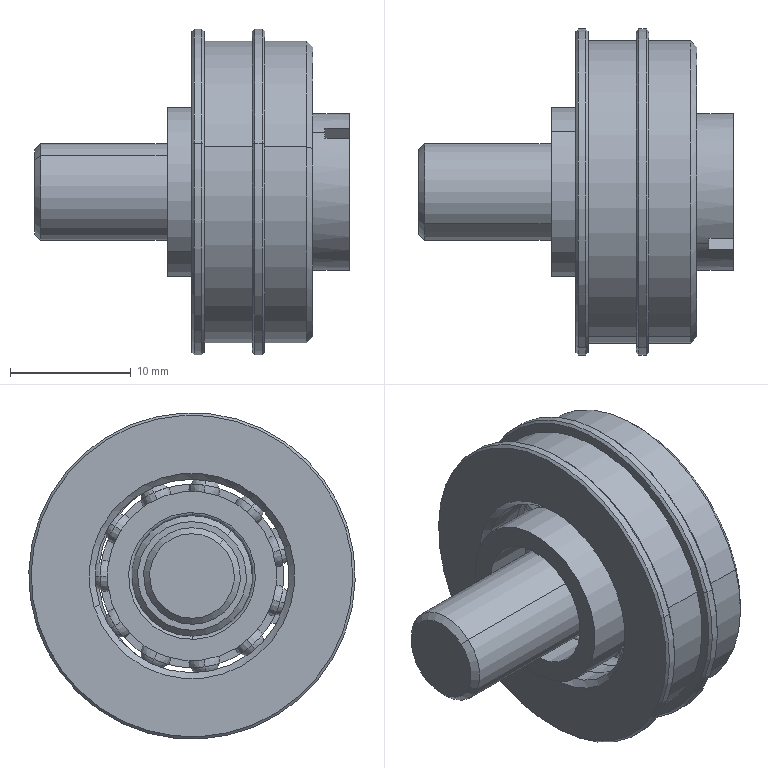Part | SolidWorks | 5 solids | 258 faces | box 26 x 27 x 27 mm | volume 5259 mm3 | sphere 88 | cylinder 59 | plane 49 | torus 44 | cone 18 | commonest cylinder face diameters 19 x6 2 x4 10 x4 12.6 x4 16.4 x4 25 x4